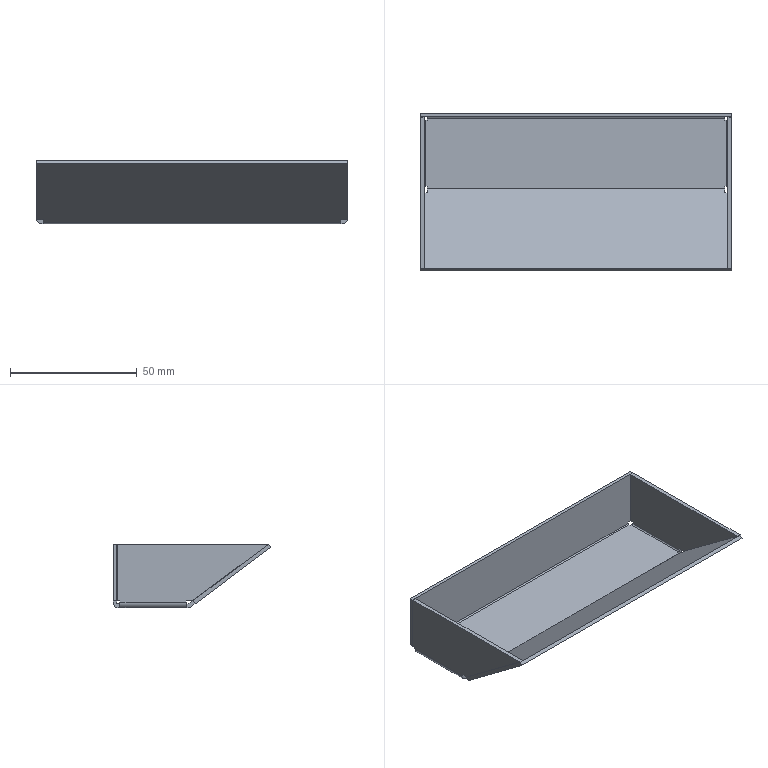Part | STEP file | Rear Closing Plate Handle | 1 solid | 46 faces | box 123 x 62.38 x 25 mm | volume 20088 mm3 | plane 38 | cylinder 8 | commonest cylinder face diameters 1 x4 4 x4
STEP:
#1=CARTESIAN_POINT('',(96.195,-17.121,0.3947));
#2=VERTEX_POINT('',#1);
#3=CARTESIAN_POINT('',(-21.305,-17.121,0.3947));
#4=VERTEX_POINT('',#3);
#5=CARTESIAN_POINT('',(-24.055,-17.121,0.3947));
#6=DIRECTION('',(-1.,0.,0.));
#7=VECTOR('',#6,1000.);
#8=LINE('',#5,#7);
#9=EDGE_CURVE('',#2,#4,#8,.T.);
#10=ORIENTED_EDGE('',*,*,#9,.F.);
#11=CARTESIAN_POINT('',(96.195,-18.621,1.51));
#12=VERTEX_POINT('',#11);
#13=CARTESIAN_POINT('',(96.195,-16.589,0.));
#14=DIRECTION('',(0.,0.8026,-0.5965));
#15=VECTOR('',#14,1000.);
#16=LINE('',#13,#15);
#17=EDGE_CURVE('',#12,#2,#16,.T.);
#18=ORIENTED_EDGE('',*,*,#17,.F.);
#19=CARTESIAN_POINT('',(98.945,-18.621,1.51));
#20=VERTEX_POINT('',#19);
#21=CARTESIAN_POINT('',(-24.055,-18.621,1.51));
#22=DIRECTION('',(-1.,0.,0.));
#23=VECTOR('',#22,1000.);
#24=LINE('',#21,#23);
#25=EDGE_CURVE('',#20,#12,#24,.T.);
#26=ORIENTED_EDGE('',*,*,#25,.F.);
#27=CARTESIAN_POINT('',(98.945,-48.612,23.796));
#28=VERTEX_POINT('',#27);
#29=CARTESIAN_POINT('',(98.945,-16.589,0.));
#30=DIRECTION('',(0.,0.8026,-0.5965));
#31=VECTOR('',#30,1000.);
#32=LINE('',#29,#31);
#33=EDGE_CURVE('',#28,#20,#32,.T.);
#34=ORIENTED_EDGE('',*,*,#33,.F.);
#35=CARTESIAN_POINT('',(-24.055,-48.612,23.796));
#36=VERTEX_POINT('',#35);
#37=CARTESIAN_POINT('',(-24.055,-48.612,23.796));
#38=DIRECTION('',(1.,0.,0.));
#39=VECTOR('',#38,1000.);
#40=LINE('',#37,#39);
#41=EDGE_CURVE('',#36,#28,#40,.T.);
#42=ORIENTED_EDGE('',*,*,#41,.F.);
#43=CARTESIAN_POINT('',(-24.055,-18.621,1.51));
#44=VERTEX_POINT('',#43);
#45=CARTESIAN_POINT('',(-24.055,-16.589,0.));
#46=DIRECTION('',(0.,-0.8026,0.5965));
#47=VECTOR('',#46,1000.);
#48=LINE('',#45,#47);
#49=EDGE_CURVE('',#44,#36,#48,.T.);
#50=ORIENTED_EDGE('',*,*,#49,.F.);
#51=CARTESIAN_POINT('',(-21.305,-18.621,1.51));
#52=VERTEX_POINT('',#51);
#53=CARTESIAN_POINT('',(-24.055,-18.621,1.51));
#54=DIRECTION('',(-1.,0.,0.));
#55=VECTOR('',#54,1000.);
#56=LINE('',#53,#55);
#57=EDGE_CURVE('',#52,#44,#56,.T.);
#58=ORIENTED_EDGE('',*,*,#57,.F.);
#59=CARTESIAN_POINT('',(-21.305,-16.589,0.));
#60=DIRECTION('',(0.,-0.8026,0.5965));
#61=VECTOR('',#60,1000.);
#62=LINE('',#59,#61);
#63=EDGE_CURVE('',#4,#52,#62,.T.);
#64=ORIENTED_EDGE('',*,*,#63,.F.);
#65=EDGE_LOOP('',(#10,#18,#26,#34,#42,#50,#58,#64));
#66=FACE_OUTER_BOUND('',#65,.T.);
#67=CARTESIAN_POINT('',(-24.055,-16.589,0.));
#68=DIRECTION('',(0.,0.5965,0.8026));
#69=DIRECTION('',(0.,-0.8026,0.5965));
#70=AXIS2_PLACEMENT_3D('',#67,#68,#69);
#71=PLANE('',#70);
#72=ADVANCED_FACE('',(#66),#71,.F.);
#73=CARTESIAN_POINT('',(-21.305,-17.727,2.714));
#74=VERTEX_POINT('',#73);
#75=CARTESIAN_POINT('',(-21.305,-16.226,1.599));
#76=VERTEX_POINT('',#75);
#77=CARTESIAN_POINT('',(-21.305,-17.727,2.714));
#78=DIRECTION('',(0.,0.8026,-0.5965));
#79=VECTOR('',#78,1000.);
#80=LINE('',#77,#79);
#81=EDGE_CURVE('',#74,#76,#80,.T.);
#82=ORIENTED_EDGE('',*,*,#81,.T.);
#83=CARTESIAN_POINT('',(-21.305,-15.928,1.5));
#84=VERTEX_POINT('',#83);
#85=CARTESIAN_POINT('',(-21.305,-15.928,2.));
#86=DIRECTION('',(1.,0.,0.));
#87=DIRECTION('',(0.,0.,-1.));
#88=AXIS2_PLACEMENT_3D('',#85,#86,#87);
#89=CIRCLE('',#88,0.5);
#90=EDGE_CURVE('',#76,#84,#89,.T.);
#91=ORIENTED_EDGE('',*,*,#90,.T.);
#92=CARTESIAN_POINT('',(-21.305,-15.178,1.5));
#93=VERTEX_POINT('',#92);
#94=CARTESIAN_POINT('',(-21.305,0.,1.5));
#95=DIRECTION('',(0.,-1.,0.));
#96=VECTOR('',#95,1000.);
#97=LINE('',#94,#96);
#98=EDGE_CURVE('',#93,#84,#97,.T.);
#99=ORIENTED_EDGE('',*,*,#98,.F.);
#100=CARTESIAN_POINT('',(-21.305,-15.178,0.));
#101=VERTEX_POINT('',#100);
#102=CARTESIAN_POINT('',(-21.305,-15.178,245.861));
#103=DIRECTION('',(0.,0.,-1.));
#104=VECTOR('',#103,1000.);
#105=LINE('',#102,#104);
#106=EDGE_CURVE('',#93,#101,#105,.T.);
#107=ORIENTED_EDGE('',*,*,#106,.T.);
#108=CARTESIAN_POINT('',(-21.305,-15.928,0.));
#109=VERTEX_POINT('',#108);
#110=CARTESIAN_POINT('',(-21.305,0.,0.));
#111=DIRECTION('',(0.,-1.,0.));
#112=VECTOR('',#111,1000.);
#113=LINE('',#110,#112);
#114=EDGE_CURVE('',#101,#109,#113,.T.);
#115=ORIENTED_EDGE('',*,*,#114,.T.);
#116=CARTESIAN_POINT('',(-21.305,-15.928,2.));
#117=DIRECTION('',(1.,0.,0.));
#118=DIRECTION('',(0.,0.,-1.));
#119=AXIS2_PLACEMENT_3D('',#116,#117,#118);
#120=CIRCLE('',#119,2.);
#121=EDGE_CURVE('',#4,#109,#120,.T.);
#122=ORIENTED_EDGE('',*,*,#121,.F.);
#123=ORIENTED_EDGE('',*,*,#63,.T.);
#124=CARTESIAN_POINT('',(-21.305,-18.621,1.51));
#125=DIRECTION('',(0.,0.5965,0.8026));
#126=VECTOR('',#125,1000.);
#127=LINE('',#124,#126);
#128=EDGE_CURVE('',#52,#74,#127,.T.);
#129=ORIENTED_EDGE('',*,*,#128,.T.);
#130=EDGE_LOOP('',(#82,#91,#99,#107,#115,#122,#123,#129));
#131=FACE_OUTER_BOUND('',#130,.T.);
#132=CARTESIAN_POINT('',(-21.305,138.317,208.457));
#133=DIRECTION('',(-1.,0.,0.));
#134=DIRECTION('',(0.,0.,1.));
#135=AXIS2_PLACEMENT_3D('',#132,#133,#134);
#136=PLANE('',#135);
#137=ADVANCED_FACE('',(#131),#136,.T.);
#138=CARTESIAN_POINT('',(96.195,-15.928,0.));
#139=VERTEX_POINT('',#138);
#140=CARTESIAN_POINT('',(96.195,-15.928,2.));
#141=DIRECTION('',(-1.,0.,0.));
#142=DIRECTION('',(0.,0.,-1.));
#143=AXIS2_PLACEMENT_3D('',#140,#141,#142);
#144=CIRCLE('',#143,2.);
#145=EDGE_CURVE('',#139,#2,#144,.T.);
#146=ORIENTED_EDGE('',*,*,#145,.T.);
#147=ORIENTED_EDGE('',*,*,#9,.T.);
#148=ORIENTED_EDGE('',*,*,#121,.T.);
#149=CARTESIAN_POINT('',(-164.795,-15.928,0.));
#150=DIRECTION('',(1.,0.,0.));
#151=VECTOR('',#150,1000.);
#152=LINE('',#149,#151);
#153=EDGE_CURVE('',#109,#139,#152,.T.);
#154=ORIENTED_EDGE('',*,*,#153,.T.);
#155=EDGE_LOOP('',(#146,#147,#148,#154));
#156=FACE_OUTER_BOUND('',#155,.T.);
#157=CARTESIAN_POINT('',(-164.795,-15.928,2.));
#158=DIRECTION('',(1.,0.,0.));
#159=DIRECTION('',(0.,0.,-1.));
#160=AXIS2_PLACEMENT_3D('',#157,#158,#159);
#161=CYLINDRICAL_SURFACE('',#160,2.);
#162=ADVANCED_FACE('',(#156),#161,.T.);
#163=CARTESIAN_POINT('',(96.195,-16.226,1.599));
#164=VERTEX_POINT('',#163);
#165=CARTESIAN_POINT('',(96.195,-17.727,2.714));
#166=VERTEX_POINT('',#165);
#167=CARTESIAN_POINT('',(96.195,-16.226,1.599));
#168=DIRECTION('',(0.,-0.8026,0.5965));
#169=VECTOR('',#168,1000.);
#170=LINE('',#167,#169);
#171=EDGE_CURVE('',#164,#166,#170,.T.);
#172=ORIENTED_EDGE('',*,*,#171,.T.);
#173=CARTESIAN_POINT('',(96.195,-17.727,2.714));
#174=DIRECTION('',(0.,-0.5965,-0.8026));
#175=VECTOR('',#174,1000.);
#176=LINE('',#173,#175);
#177=EDGE_CURVE('',#166,#12,#176,.T.);
#178=ORIENTED_EDGE('',*,*,#177,.T.);
#179=ORIENTED_EDGE('',*,*,#17,.T.);
#180=ORIENTED_EDGE('',*,*,#145,.F.);
#181=CARTESIAN_POINT('',(96.195,-15.178,0.));
#182=VERTEX_POINT('',#181);
#183=CARTESIAN_POINT('',(96.195,0.,0.));
#184=DIRECTION('',(0.,1.,0.));
#185=VECTOR('',#184,1000.);
#186=LINE('',#183,#185);
#187=EDGE_CURVE('',#139,#182,#186,.T.);
#188=ORIENTED_EDGE('',*,*,#187,.T.);
#189=CARTESIAN_POINT('',(96.195,-15.178,1.5));
#190=VERTEX_POINT('',#189);
#191=CARTESIAN_POINT('',(96.195,-15.178,245.861));
#192=DIRECTION('',(0.,0.,1.));
#193=VECTOR('',#192,1000.);
#194=LINE('',#191,#193);
#195=EDGE_CURVE('',#182,#190,#194,.T.);
#196=ORIENTED_EDGE('',*,*,#195,.T.);
#197=CARTESIAN_POINT('',(96.195,-15.928,1.5));
#198=VERTEX_POINT('',#197);
#199=CARTESIAN_POINT('',(96.195,0.,1.5));
#200=DIRECTION('',(0.,-1.,0.));
#201=VECTOR('',#200,1000.);
#202=LINE('',#199,#201);
#203=EDGE_CURVE('',#190,#198,#202,.T.);
#204=ORIENTED_EDGE('',*,*,#203,.T.);
#205=CARTESIAN_POINT('',(96.195,-15.928,2.));
#206=DIRECTION('',(-1.,0.,0.));
#207=DIRECTION('',(0.,0.,-1.));
#208=AXIS2_PLACEMENT_3D('',#205,#206,#207);
#209=CIRCLE('',#208,0.5);
#210=EDGE_CURVE('',#198,#164,#209,.T.);
#211=ORIENTED_EDGE('',*,*,#210,.T.);
#212=EDGE_LOOP('',(#172,#178,#179,#180,#188,#196,#204,#211));
#213=FACE_OUTER_BOUND('',#212,.T.);
#214=CARTESIAN_POINT('',(96.195,138.317,208.457));
#215=DIRECTION('',(1.,0.,0.));
#216=DIRECTION('',(0.,0.,-1.));
#217=AXIS2_PLACEMENT_3D('',#214,#215,#216);
#218=PLANE('',#217);
#219=ADVANCED_FACE('',(#213),#218,.T.);
#220=CARTESIAN_POINT('',(98.945,-17.727,2.714));
#221=VERTEX_POINT('',#220);
#222=CARTESIAN_POINT('',(-24.055,-17.727,2.714));
#223=DIRECTION('',(1.,0.,0.));
#224=VECTOR('',#223,1000.);
#225=LINE('',#222,#224);
#226=EDGE_CURVE('',#166,#221,#225,.T.);
#227=ORIENTED_EDGE('',*,*,#226,.T.);
#228=CARTESIAN_POINT('',(98.945,136.285,209.967));
#229=DIRECTION('',(0.,-0.5965,-0.8026));
#230=VECTOR('',#229,1000.);
#231=LINE('',#228,#230);
#232=EDGE_CURVE('',#221,#20,#231,.T.);
#233=ORIENTED_EDGE('',*,*,#232,.T.);
#234=ORIENTED_EDGE('',*,*,#25,.T.);
#235=ORIENTED_EDGE('',*,*,#177,.F.);
#236=EDGE_LOOP('',(#227,#233,#234,#235));
#237=FACE_OUTER_BOUND('',#236,.T.);
#238=CARTESIAN_POINT('',(-24.055,136.285,209.967));
#239=DIRECTION('',(0.,0.8026,-0.5965));
#240=DIRECTION('',(0.,0.5965,0.8026));
#241=AXIS2_PLACEMENT_3D('',#238,#239,#240);
#242=PLANE('',#241);
#243=ADVANCED_FACE('',(#237),#242,.T.);
#244=ORIENTED_EDGE('',*,*,#33,.T.);
#245=ORIENTED_EDGE('',*,*,#232,.F.);
#246=CARTESIAN_POINT('',(98.945,-47.717,25.));
#247=VERTEX_POINT('',#246);
#248=CARTESIAN_POINT('',(98.945,-47.717,25.));
#249=DIRECTION('',(0.,0.8026,-0.5965));
#250=VECTOR('',#249,1000.);
#251=LINE('',#248,#250);
#252=EDGE_CURVE('',#247,#221,#251,.T.);
#253=ORIENTED_EDGE('',*,*,#252,.F.);
#254=CARTESIAN_POINT('',(98.945,-48.612,23.796));
#255=DIRECTION('',(0.,0.5965,0.8026));
#256=VECTOR('',#255,1000.);
#257=LINE('',#254,#256);
#258=EDGE_CURVE('',#28,#247,#257,.T.);
#259=ORIENTED_EDGE('',*,*,#258,.F.);
#260=EDGE_LOOP('',(#244,#245,#253,#259));
#261=FACE_OUTER_BOUND('',#260,.T.);
#262=CARTESIAN_POINT('',(98.945,88.075,245.792));
#263=DIRECTION('',(-1.,0.,0.));
#264=DIRECTION('',(0.,-1.,0.));
#265=AXIS2_PLACEMENT_3D('',#262,#263,#264);
#266=PLANE('',#265);
#267=ADVANCED_FACE('',(#261),#266,.F.);
#268=ORIENTED_EDGE('',*,*,#41,.T.);
#269=ORIENTED_EDGE('',*,*,#258,.T.);
#270=CARTESIAN_POINT('',(-24.055,-47.717,25.));
#271=VERTEX_POINT('',#270);
#272=CARTESIAN_POINT('',(-24.055,-47.717,25.));
#273=DIRECTION('',(1.,0.,0.));
#274=VECTOR('',#273,1000.);
#275=LINE('',#272,#274);
#276=EDGE_CURVE('',#271,#247,#275,.T.);
#277=ORIENTED_EDGE('',*,*,#276,.F.);
#278=CARTESIAN_POINT('',(-24.055,106.295,232.253));
#279=DIRECTION('',(0.,0.5965,0.8026));
#280=VECTOR('',#279,1000.);
#281=LINE('',#278,#280);
#282=EDGE_CURVE('',#36,#271,#281,.T.);
#283=ORIENTED_EDGE('',*,*,#282,.F.);
#284=EDGE_LOOP('',(#268,#269,#277,#283));
#285=FACE_OUTER_BOUND('',#284,.T.);
#286=CARTESIAN_POINT('',(-24.055,106.295,232.253));
#287=DIRECTION('',(0.,0.8026,-0.5965));
#288=DIRECTION('',(0.,0.5965,0.8026));
#289=AXIS2_PLACEMENT_3D('',#286,#287,#288);
#290=PLANE('',#289);
#291=ADVANCED_FACE('',(#285),#290,.F.);
#292=ORIENTED_EDGE('',*,*,#49,.T.);
#293=ORIENTED_EDGE('',*,*,#282,.T.);
#294=CARTESIAN_POINT('',(-24.055,-17.727,2.714));
#295=VERTEX_POINT('',#294);
#296=CARTESIAN_POINT('',(-24.055,-17.727,2.714));
#297=DIRECTION('',(0.,-0.8026,0.5965));
#298=VECTOR('',#297,1000.);
#299=LINE('',#296,#298);
#300=EDGE_CURVE('',#295,#271,#299,.T.);
#301=ORIENTED_EDGE('',*,*,#300,.F.);
#302=CARTESIAN_POINT('',(-24.055,-18.621,1.51));
#303=DIRECTION('',(0.,0.5965,0.8026));
#304=VECTOR('',#303,1000.);
#305=LINE('',#302,#304);
#306=EDGE_CURVE('',#44,#295,#305,.T.);
#307=ORIENTED_EDGE('',*,*,#306,.F.);
#308=EDGE_LOOP('',(#292,#293,#301,#307));
#309=FACE_OUTER_BOUND('',#308,.T.);
#310=CARTESIAN_POINT('',(-24.055,156.138,195.213));
#311=DIRECTION('',(1.,0.,0.));
#312=DIRECTION('',(0.,0.,-1.));
#313=AXIS2_PLACEMENT_3D('',#310,#311,#312);
#314=PLANE('',#313);
#315=ADVANCED_FACE('',(#309),#314,.F.);
#316=CARTESIAN_POINT('',(-24.055,-17.727,2.714));
#317=DIRECTION('',(1.,0.,0.));
#318=VECTOR('',#317,1000.);
#319=LINE('',#316,#318);
#320=EDGE_CURVE('',#295,#74,#319,.T.);
#321=ORIENTED_EDGE('',*,*,#320,.T.);
#322=ORIENTED_EDGE('',*,*,#128,.F.);
#323=ORIENTED_EDGE('',*,*,#57,.T.);
#324=ORIENTED_EDGE('',*,*,#306,.T.);
#325=EDGE_LOOP('',(#321,#322,#323,#324));
#326=FACE_OUTER_BOUND('',#325,.T.);
#327=CARTESIAN_POINT('',(-24.055,136.285,209.967));
#328=DIRECTION('',(0.,0.8026,-0.5965));
#329=DIRECTION('',(0.,0.5965,0.8026));
#330=AXIS2_PLACEMENT_3D('',#327,#328,#329);
#331=PLANE('',#330);
#332=ADVANCED_FACE('',(#326),#331,.T.);
#333=CARTESIAN_POINT('',(-24.055,-16.226,1.599));
#334=DIRECTION('',(-1.,0.,0.));
#335=VECTOR('',#334,1000.);
#336=LINE('',#333,#335);
#337=EDGE_CURVE('',#164,#76,#336,.T.);
#338=ORIENTED_EDGE('',*,*,#337,.T.);
#339=ORIENTED_EDGE('',*,*,#81,.F.);
#340=ORIENTED_EDGE('',*,*,#320,.F.);
#341=ORIENTED_EDGE('',*,*,#300,.T.);
#342=ORIENTED_EDGE('',*,*,#276,.T.);
#343=ORIENTED_EDGE('',*,*,#252,.T.);
#344=ORIENTED_EDGE('',*,*,#226,.F.);
#345=ORIENTED_EDGE('',*,*,#171,.F.);
#346=EDGE_LOOP('',(#338,#339,#340,#341,#342,#343,#344,#345));
#347=FACE_OUTER_BOUND('',#346,.T.);
#348=CARTESIAN_POINT('',(-24.055,-15.695,1.204));
#349=DIRECTION('',(0.,0.5965,0.8026));
#350=DIRECTION('',(0.,-0.8026,0.5965));
#351=AXIS2_PLACEMENT_3D('',#348,#349,#350);
#352=PLANE('',#351);
#353=ADVANCED_FACE('',(#347),#352,.T.);
#354=ORIENTED_EDGE('',*,*,#114,.F.);
#355=CARTESIAN_POINT('',(-22.055,-15.178,0.));
#356=VERTEX_POINT('',#355);
#357=CARTESIAN_POINT('',(0.,-15.178,0.));
#358=DIRECTION('',(1.,0.,0.));
#359=VECTOR('',#358,1000.);
#360=LINE('',#357,#359);
#361=EDGE_CURVE('',#356,#101,#360,.T.);
#362=ORIENTED_EDGE('',*,*,#361,.F.);
#363=CARTESIAN_POINT('',(-22.055,11.018,0.));
#364=VERTEX_POINT('',#363);
#365=CARTESIAN_POINT('',(-22.055,0.,0.));
#366=DIRECTION('',(0.,-1.,0.));
#367=VECTOR('',#366,1000.);
#368=LINE('',#365,#367);
#369=EDGE_CURVE('',#364,#356,#368,.T.);
#370=ORIENTED_EDGE('',*,*,#369,.F.);
#371=CARTESIAN_POINT('',(-21.305,11.018,0.));
#372=VERTEX_POINT('',#371);
#373=CARTESIAN_POINT('',(0.,11.018,0.));
#374=DIRECTION('',(-1.,0.,0.));
#375=VECTOR('',#374,1000.);
#376=LINE('',#373,#375);
#377=EDGE_CURVE('',#372,#364,#376,.T.);
#378=ORIENTED_EDGE('',*,*,#377,.F.);
#379=CARTESIAN_POINT('',(-21.305,11.768,0.));
#380=VERTEX_POINT('',#379);
#381=CARTESIAN_POINT('',(-21.305,0.,0.));
#382=DIRECTION('',(0.,1.,0.));
#383=VECTOR('',#382,1000.);
#384=LINE('',#381,#383);
#385=EDGE_CURVE('',#372,#380,#384,.T.);
#386=ORIENTED_EDGE('',*,*,#385,.T.);
#387=CARTESIAN_POINT('',(96.195,11.768,0.));
#388=VERTEX_POINT('',#387);
#389=CARTESIAN_POINT('',(0.,11.768,0.));
#390=DIRECTION('',(-1.,0.,0.));
#391=VECTOR('',#390,1000.);
#392=LINE('',#389,#391);
#393=EDGE_CURVE('',#388,#380,#392,.T.);
#394=ORIENTED_EDGE('',*,*,#393,.F.);
#395=CARTESIAN_POINT('',(96.195,11.018,0.));
#396=VERTEX_POINT('',#395);
#397=CARTESIAN_POINT('',(96.195,0.,0.));
#398=DIRECTION('',(0.,-1.,0.));
#399=VECTOR('',#398,1000.);
#400=LINE('',#397,#399);
#401=EDGE_CURVE('',#388,#396,#400,.T.);
#402=ORIENTED_EDGE('',*,*,#401,.T.);
#403=CARTESIAN_POINT('',(96.945,11.018,0.));
#404=VERTEX_POINT('',#403);
#405=CARTESIAN_POINT('',(0.,11.018,0.));
#406=DIRECTION('',(-1.,0.,0.));
#407=VECTOR('',#406,1000.);
#408=LINE('',#405,#407);
#409=EDGE_CURVE('',#404,#396,#408,.T.);
#410=ORIENTED_EDGE('',*,*,#409,.F.);
#411=CARTESIAN_POINT('',(96.945,-15.178,0.));
#412=VERTEX_POINT('',#411);
#413=CARTESIAN_POINT('',(96.945,0.,0.));
#414=DIRECTION('',(0.,1.,0.));
#415=VECTOR('',#414,1000.);
#416=LINE('',#413,#415);
#417=EDGE_CURVE('',#412,#404,#416,.T.);
#418=ORIENTED_EDGE('',*,*,#417,.F.);
#419=CARTESIAN_POINT('',(0.,-15.178,0.));
#420=DIRECTION('',(1.,0.,0.));
#421=VECTOR('',#420,1000.);
#422=LINE('',#419,#421);
#423=EDGE_CURVE('',#182,#412,#422,.T.);
#424=ORIENTED_EDGE('',*,*,#423,.F.);
#425=ORIENTED_EDGE('',*,*,#187,.F.);
#426=ORIENTED_EDGE('',*,*,#153,.F.);
#427=EDGE_LOOP('',(#354,#362,#370,#378,#386,#394,#402,#410,#418,#424,#425,#426));
#428=FACE_OUTER_BOUND('',#427,.T.);
#429=CARTESIAN_POINT('',(0.,0.,0.));
#430=DIRECTION('',(0.,0.,1.));
#431=DIRECTION('',(1.,0.,0.));
#432=AXIS2_PLACEMENT_3D('',#429,#430,#431);
#433=PLANE('',#432);
#434=ADVANCED_FACE('',(#428),#433,.F.);
#435=ORIENTED_EDGE('',*,*,#337,.F.);
#436=ORIENTED_EDGE('',*,*,#210,.F.);
#437=CARTESIAN_POINT('',(-164.795,-15.928,1.5));
#438=DIRECTION('',(1.,0.,0.));
#439=VECTOR('',#438,1000.);
#440=LINE('',#437,#439);
#441=EDGE_CURVE('',#84,#198,#440,.T.);
#442=ORIENTED_EDGE('',*,*,#441,.F.);
#443=ORIENTED_EDGE('',*,*,#90,.F.);
#444=EDGE_LOOP('',(#435,#436,#442,#443));
#445=FACE_OUTER_BOUND('',#444,.T.);
#446=CARTESIAN_POINT('',(-164.795,-15.928,2.));
#447=DIRECTION('',(1.,0.,0.));
#448=DIRECTION('',(0.,0.,-1.));
#449=AXIS2_PLACEMENT_3D('',#446,#447,#448);
#450=CYLINDRICAL_SURFACE('',#449,0.5);
#451=ADVANCED_FACE('',(#445),#450,.F.);
#452=CARTESIAN_POINT('',(-22.055,-15.178,1.5));
#453=VERTEX_POINT('',#452);
#454=CARTESIAN_POINT('',(0.,-15.178,1.5));
#455=DIRECTION('',(-1.,0.,0.));
#456=VECTOR('',#455,1000.);
#457=LINE('',#454,#456);
#458=EDGE_CURVE('',#93,#453,#457,.T.);
#459=ORIENTED_EDGE('',*,*,#458,.T.);
#460=CARTESIAN_POINT('',(-22.555,-15.178,2.));
#461=VERTEX_POINT('',#460);
#462=CARTESIAN_POINT('',(-22.055,-15.178,2.));
#463=DIRECTION('',(0.,1.,0.));
#464=DIRECTION('',(0.,0.,-1.));
#465=AXIS2_PLACEMENT_3D('',#462,#463,#464);
#466=CIRCLE('',#465,0.5);
#467=EDGE_CURVE('',#453,#461,#466,.T.);
#468=ORIENTED_EDGE('',*,*,#467,.T.);
#469=CARTESIAN_POINT('',(-22.555,-15.178,2.75));
#470=VERTEX_POINT('',#469);
#471=CARTESIAN_POINT('',(-22.555,-15.178,25.));
#472=DIRECTION('',(0.,0.,1.));
#473=VECTOR('',#472,1000.);
#474=LINE('',#471,#473);
#475=EDGE_CURVE('',#461,#470,#474,.T.);
#476=ORIENTED_EDGE('',*,*,#475,.T.);
#477=CARTESIAN_POINT('',(-24.055,-15.178,2.75));
#478=VERTEX_POINT('',#477);
#479=CARTESIAN_POINT('',(105.432,-15.178,2.75));
#480=DIRECTION('',(1.,0.,0.));
#481=VECTOR('',#480,1000.);
#482=LINE('',#479,#481);
#483=EDGE_CURVE('',#478,#470,#482,.T.);
#484=ORIENTED_EDGE('',*,*,#483,.F.);
#485=CARTESIAN_POINT('',(-24.055,-15.178,2.));
#486=VERTEX_POINT('',#485);
#487=CARTESIAN_POINT('',(-24.055,-15.178,25.));
#488=DIRECTION('',(0.,0.,-1.));
#489=VECTOR('',#488,1000.);
#490=LINE('',#487,#489);
#491=EDGE_CURVE('',#478,#486,#490,.T.);
#492=ORIENTED_EDGE('',*,*,#491,.T.);
#493=CARTESIAN_POINT('',(-22.055,-15.178,2.));
#494=DIRECTION('',(0.,1.,0.));
#495=DIRECTION('',(0.,0.,-1.));
#496=AXIS2_PLACEMENT_3D('',#493,#494,#495);
#497=CIRCLE('',#496,2.);
#498=EDGE_CURVE('',#356,#486,#497,.T.);
#499=ORIENTED_EDGE('',*,*,#498,.F.);
#500=ORIENTED_EDGE('',*,*,#361,.T.);
#501=ORIENTED_EDGE('',*,*,#106,.F.);
#502=EDGE_LOOP('',(#459,#468,#476,#484,#492,#499,#500,#501));
#503=FACE_OUTER_BOUND('',#502,.T.);
#504=CARTESIAN_POINT('',(0.,-15.178,245.861));
#505=DIRECTION('',(0.,-1.,0.));
#506=DIRECTION('',(1.,0.,0.));
#507=AXIS2_PLACEMENT_3D('',#504,#505,#506);
#508=PLANE('',#507);
#509=ADVANCED_FACE('',(#503),#508,.T.);
#510=ORIENTED_EDGE('',*,*,#498,.T.);
#511=CARTESIAN_POINT('',(-24.055,11.018,2.));
#512=VERTEX_POINT('',#511);
#513=CARTESIAN_POINT('',(-24.055,174.2,2.));
#514=DIRECTION('',(0.,1.,0.));
#515=VECTOR('',#514,1000.);
#516=LINE('',#513,#515);
#517=EDGE_CURVE('',#486,#512,#516,.T.);
#518=ORIENTED_EDGE('',*,*,#517,.T.);
#519=CARTESIAN_POINT('',(-22.055,11.018,2.));
#520=DIRECTION('',(0.,-1.,0.));
#521=DIRECTION('',(0.,0.,-1.));
#522=AXIS2_PLACEMENT_3D('',#519,#520,#521);
#523=CIRCLE('',#522,2.);
#524=EDGE_CURVE('',#512,#364,#523,.T.);
#525=ORIENTED_EDGE('',*,*,#524,.T.);
#526=ORIENTED_EDGE('',*,*,#369,.T.);
#527=EDGE_LOOP('',(#510,#518,#525,#526));
#528=FACE_OUTER_BOUND('',#527,.T.);
#529=CARTESIAN_POINT('',(-22.055,174.2,2.));
#530=DIRECTION('',(0.,-1.,0.));
#531=DIRECTION('',(0.,0.,-1.));
#532=AXIS2_PLACEMENT_3D('',#529,#530,#531);
#533=CYLINDRICAL_SURFACE('',#532,2.);
#534=ADVANCED_FACE('',(#528),#533,.T.);
#535=ORIENTED_EDGE('',*,*,#377,.T.);
#536=ORIENTED_EDGE('',*,*,#524,.F.);
#537=CARTESIAN_POINT('',(-24.055,11.018,2.75));
#538=VERTEX_POINT('',#537);
#539=CARTESIAN_POINT('',(-24.055,11.018,25.));
#540=DIRECTION('',(0.,0.,1.));
#541=VECTOR('',#540,1000.);
#542=LINE('',#539,#541);
#543=EDGE_CURVE('',#512,#538,#542,.T.);
#544=ORIENTED_EDGE('',*,*,#543,.T.);
#545=CARTESIAN_POINT('',(-22.555,11.018,2.75));
#546=VERTEX_POINT('',#545);
#547=CARTESIAN_POINT('',(105.432,11.018,2.75));
#548=DIRECTION('',(-1.,0.,0.));
#549=VECTOR('',#548,1000.);
#550=LINE('',#547,#549);
#551=EDGE_CURVE('',#546,#538,#550,.T.);
#552=ORIENTED_EDGE('',*,*,#551,.F.);
#553=CARTESIAN_POINT('',(-22.555,11.018,2.));
#554=VERTEX_POINT('',#553);
#555=CARTESIAN_POINT('',(-22.555,11.018,25.));
#556=DIRECTION('',(0.,0.,1.));
#557=VECTOR('',#556,1000.);
#558=LINE('',#555,#557);
#559=EDGE_CURVE('',#554,#546,#558,.T.);
#560=ORIENTED_EDGE('',*,*,#559,.F.);
#561=CARTESIAN_POINT('',(-22.055,11.018,1.5));
#562=VERTEX_POINT('',#561);
#563=CARTESIAN_POINT('',(-22.055,11.018,2.));
#564=DIRECTION('',(0.,-1.,0.));
#565=DIRECTION('',(0.,0.,-1.));
#566=AXIS2_PLACEMENT_3D('',#563,#564,#565);
#567=CIRCLE('',#566,0.5);
#568=EDGE_CURVE('',#554,#562,#567,.T.);
#569=ORIENTED_EDGE('',*,*,#568,.T.);
#570=CARTESIAN_POINT('',(-21.305,11.018,1.5));
#571=VERTEX_POINT('',#570);
#572=CARTESIAN_POINT('',(0.,11.018,1.5));
#573=DIRECTION('',(-1.,0.,0.));
#574=VECTOR('',#573,1000.);
#575=LINE('',#572,#574);
#576=EDGE_CURVE('',#571,#562,#575,.T.);
#577=ORIENTED_EDGE('',*,*,#576,.F.);
#578=CARTESIAN_POINT('',(-21.305,11.018,245.861));
#579=DIRECTION('',(0.,0.,1.));
#580=VECTOR('',#579,1000.);
#581=LINE('',#578,#580);
#582=EDGE_CURVE('',#372,#571,#581,.T.);
#583=ORIENTED_EDGE('',*,*,#582,.F.);
#584=EDGE_LOOP('',(#535,#536,#544,#552,#560,#569,#577,#583));
#585=FACE_OUTER_BOUND('',#584,.T.);
#586=CARTESIAN_POINT('',(0.,11.018,245.861));
#587=DIRECTION('',(0.,-1.,0.));
#588=DIRECTION('',(0.,0.,-1.));
#589=AXIS2_PLACEMENT_3D('',#586,#587,#588);
#590=PLANE('',#589);
#591=ADVANCED_FACE('',(#585),#590,.F.);
#592=CARTESIAN_POINT('',(-21.305,13.768,2.));
#593=VERTEX_POINT('',#592);
#594=CARTESIAN_POINT('',(-21.305,11.768,2.));
#595=DIRECTION('',(1.,0.,0.));
#596=DIRECTION('',(0.,0.,1.));
#597=AXIS2_PLACEMENT_3D('',#594,#595,#596);
#598=CIRCLE('',#597,2.);
#599=EDGE_CURVE('',#380,#593,#598,.T.);
#600=ORIENTED_EDGE('',*,*,#599,.T.);
#601=CARTESIAN_POINT('',(96.195,13.768,2.));
#602=VERTEX_POINT('',#601);
#603=CARTESIAN_POINT('',(287.743,13.768,2.));
#604=DIRECTION('',(1.,0.,0.));
#605=VECTOR('',#604,1000.);
#606=LINE('',#603,#605);
#607=EDGE_CURVE('',#593,#602,#606,.T.);
#608=ORIENTED_EDGE('',*,*,#607,.T.);
#609=CARTESIAN_POINT('',(96.195,11.768,2.));
#610=DIRECTION('',(-1.,0.,0.));
#611=DIRECTION('',(0.,0.,1.));
#612=AXIS2_PLACEMENT_3D('',#609,#610,#611);
#613=CIRCLE('',#612,2.);
#614=EDGE_CURVE('',#602,#388,#613,.T.);
#615=ORIENTED_EDGE('',*,*,#614,.T.);
#616=ORIENTED_EDGE('',*,*,#393,.T.);
#617=EDGE_LOOP('',(#600,#608,#615,#616));
#618=FACE_OUTER_BOUND('',#617,.T.);
#619=CARTESIAN_POINT('',(287.743,11.768,2.));
#620=DIRECTION('',(-1.,0.,0.));
#621=DIRECTION('',(0.,0.,1.));
#622=AXIS2_PLACEMENT_3D('',#619,#620,#621);
#623=CYLINDRICAL_SURFACE('',#622,2.);
#624=ADVANCED_FACE('',(#618),#623,.T.);
#625=ORIENTED_EDGE('',*,*,#409,.T.);
#626=CARTESIAN_POINT('',(96.195,11.018,1.5));
#627=VERTEX_POINT('',#626);
#628=CARTESIAN_POINT('',(96.195,11.018,245.861));
#629=DIRECTION('',(0.,0.,-1.));
#630=VECTOR('',#629,1000.);
#631=LINE('',#628,#630);
#632=EDGE_CURVE('',#627,#396,#631,.T.);
#633=ORIENTED_EDGE('',*,*,#632,.F.);
#634=CARTESIAN_POINT('',(96.945,11.018,1.5));
#635=VERTEX_POINT('',#634);
#636=CARTESIAN_POINT('',(0.,11.018,1.5));
#637=DIRECTION('',(-1.,0.,0.));
#638=VECTOR('',#637,1000.);
#639=LINE('',#636,#638);
#640=EDGE_CURVE('',#635,#627,#639,.T.);
#641=ORIENTED_EDGE('',*,*,#640,.F.);
#642=CARTESIAN_POINT('',(97.445,11.018,2.));
#643=VERTEX_POINT('',#642);
#644=CARTESIAN_POINT('',(96.945,11.018,2.));
#645=DIRECTION('',(0.,-1.,0.));
#646=DIRECTION('',(0.,0.,1.));
#647=AXIS2_PLACEMENT_3D('',#644,#645,#646);
#648=CIRCLE('',#647,0.5);
#649=EDGE_CURVE('',#635,#643,#648,.T.);
#650=ORIENTED_EDGE('',*,*,#649,.T.);
#651=CARTESIAN_POINT('',(97.445,11.018,2.75));
#652=VERTEX_POINT('',#651);
#653=CARTESIAN_POINT('',(97.445,11.018,25.));
#654=DIRECTION('',(0.,0.,-1.));
#655=VECTOR('',#654,1000.);
#656=LINE('',#653,#655);
#657=EDGE_CURVE('',#652,#643,#656,.T.);
#658=ORIENTED_EDGE('',*,*,#657,.F.);
#659=CARTESIAN_POINT('',(98.945,11.018,2.75));
#660=VERTEX_POINT('',#659);
#661=CARTESIAN_POINT('',(-30.542,11.018,2.75));
#662=DIRECTION('',(-1.,0.,0.));
#663=VECTOR('',#662,1000.);
#664=LINE('',#661,#663);
#665=EDGE_CURVE('',#660,#652,#664,.T.);
#666=ORIENTED_EDGE('',*,*,#665,.F.);
#667=CARTESIAN_POINT('',(98.945,11.018,2.));
#668=VERTEX_POINT('',#667);
#669=CARTESIAN_POINT('',(98.945,11.018,25.));
#670=DIRECTION('',(0.,0.,-1.));
#671=VECTOR('',#670,1000.);
#672=LINE('',#669,#671);
#673=EDGE_CURVE('',#660,#668,#672,.T.);
#674=ORIENTED_EDGE('',*,*,#673,.T.);
#675=CARTESIAN_POINT('',(96.945,11.018,2.));
#676=DIRECTION('',(0.,-1.,0.));
#677=DIRECTION('',(0.,0.,1.));
#678=AXIS2_PLACEMENT_3D('',#675,#676,#677);
#679=CIRCLE('',#678,2.);
#680=EDGE_CURVE('',#404,#668,#679,.T.);
#681=ORIENTED_EDGE('',*,*,#680,.F.);
#682=EDGE_LOOP('',(#625,#633,#641,#650,#658,#666,#674,#681));
#683=FACE_OUTER_BOUND('',#682,.T.);
#684=CARTESIAN_POINT('',(0.,11.018,245.861));
#685=DIRECTION('',(0.,-1.,0.));
#686=DIRECTION('',(0.,0.,-1.));
#687=AXIS2_PLACEMENT_3D('',#684,#685,#686);
#688=PLANE('',#687);
#689=ADVANCED_FACE('',(#683),#688,.F.);
#690=ORIENTED_EDGE('',*,*,#680,.T.);
#691=CARTESIAN_POINT('',(98.945,-15.178,2.));
#692=VERTEX_POINT('',#691);
#693=CARTESIAN_POINT('',(98.945,-198.697,2.));
#694=DIRECTION('',(0.,-1.,0.));
#695=VECTOR('',#694,1000.);
#696=LINE('',#693,#695);
#697=EDGE_CURVE('',#668,#692,#696,.T.);
#698=ORIENTED_EDGE('',*,*,#697,.T.);
#699=CARTESIAN_POINT('',(96.945,-15.178,2.));
#700=DIRECTION('',(0.,1.,0.));
#701=DIRECTION('',(0.,0.,1.));
#702=AXIS2_PLACEMENT_3D('',#699,#700,#701);
#703=CIRCLE('',#702,2.);
#704=EDGE_CURVE('',#692,#412,#703,.T.);
#705=ORIENTED_EDGE('',*,*,#704,.T.);
#706=ORIENTED_EDGE('',*,*,#417,.T.);
#707=EDGE_LOOP('',(#690,#698,#705,#706));
#708=FACE_OUTER_BOUND('',#707,.T.);
#709=CARTESIAN_POINT('',(96.945,-198.697,2.));
#710=DIRECTION('',(0.,1.,0.));
#711=DIRECTION('',(0.,0.,1.));
#712=AXIS2_PLACEMENT_3D('',#709,#710,#711);
#713=CYLINDRICAL_SURFACE('',#712,2.);
#714=ADVANCED_FACE('',(#708),#713,.T.);
#715=CARTESIAN_POINT('',(96.945,-15.178,1.5));
#716=VERTEX_POINT('',#715);
#717=CARTESIAN_POINT('',(0.,-15.178,1.5));
#718=DIRECTION('',(-1.,0.,0.));
#719=VECTOR('',#718,1000.);
#720=LINE('',#717,#719);
#721=EDGE_CURVE('',#716,#190,#720,.T.);
#722=ORIENTED_EDGE('',*,*,#721,.T.);
#723=ORIENTED_EDGE('',*,*,#195,.F.);
#724=ORIENTED_EDGE('',*,*,#423,.T.);
#725=ORIENTED_EDGE('',*,*,#704,.F.);
#726=CARTESIAN_POINT('',(98.945,-15.178,2.75));
#727=VERTEX_POINT('',#726);
#728=CARTESIAN_POINT('',(98.945,-15.178,25.));
#729=DIRECTION('',(0.,0.,1.));
#730=VECTOR('',#729,1000.);
#731=LINE('',#728,#730);
#732=EDGE_CURVE('',#692,#727,#731,.T.);
#733=ORIENTED_EDGE('',*,*,#732,.T.);
#734=CARTESIAN_POINT('',(97.445,-15.178,2.75));
#735=VERTEX_POINT('',#734);
#736=CARTESIAN_POINT('',(-30.542,-15.178,2.75));
#737=DIRECTION('',(1.,0.,0.));
#738=VECTOR('',#737,1000.);
#739=LINE('',#736,#738);
#740=EDGE_CURVE('',#735,#727,#739,.T.);
#741=ORIENTED_EDGE('',*,*,#740,.F.);
#742=CARTESIAN_POINT('',(97.445,-15.178,2.));
#743=VERTEX_POINT('',#742);
#744=CARTESIAN_POINT('',(97.445,-15.178,25.));
#745=DIRECTION('',(0.,0.,-1.));
#746=VECTOR('',#745,1000.);
#747=LINE('',#744,#746);
#748=EDGE_CURVE('',#735,#743,#747,.T.);
#749=ORIENTED_EDGE('',*,*,#748,.T.);
#750=CARTESIAN_POINT('',(96.945,-15.178,2.));
#751=DIRECTION('',(0.,1.,0.));
#752=DIRECTION('',(0.,0.,1.));
#753=AXIS2_PLACEMENT_3D('',#750,#751,#752);
#754=CIRCLE('',#753,0.5);
#755=EDGE_CURVE('',#743,#716,#754,.T.);
#756=ORIENTED_EDGE('',*,*,#755,.T.);
#757=EDGE_LOOP('',(#722,#723,#724,#725,#733,#741,#749,#756));
#758=FACE_OUTER_BOUND('',#757,.T.);
#759=CARTESIAN_POINT('',(0.,-15.178,245.861));
#760=DIRECTION('',(0.,-1.,0.));
#761=DIRECTION('',(0.,0.,-1.));
#762=AXIS2_PLACEMENT_3D('',#759,#760,#761);
#763=PLANE('',#762);
#764=ADVANCED_FACE('',(#758),#763,.T.);
#765=CARTESIAN_POINT('',(-22.055,0.,1.5));
#766=DIRECTION('',(0.,-1.,0.));
#767=VECTOR('',#766,1000.);
#768=LINE('',#765,#767);
#769=EDGE_CURVE('',#562,#453,#768,.T.);
#770=ORIENTED_EDGE('',*,*,#769,.T.);
#771=ORIENTED_EDGE('',*,*,#458,.F.);
#772=ORIENTED_EDGE('',*,*,#98,.T.);
#773=ORIENTED_EDGE('',*,*,#441,.T.);
#774=ORIENTED_EDGE('',*,*,#203,.F.);
#775=ORIENTED_EDGE('',*,*,#721,.F.);
#776=CARTESIAN_POINT('',(96.945,0.,1.5));
#777=DIRECTION('',(0.,1.,0.));
#778=VECTOR('',#777,1000.);
#779=LINE('',#776,#778);
#780=EDGE_CURVE('',#716,#635,#779,.T.);
#781=ORIENTED_EDGE('',*,*,#780,.T.);
#782=ORIENTED_EDGE('',*,*,#640,.T.);
#783=CARTESIAN_POINT('',(96.195,11.768,1.5));
#784=VERTEX_POINT('',#783);
#785=CARTESIAN_POINT('',(96.195,0.,1.5));
#786=DIRECTION('',(0.,1.,0.));
#787=VECTOR('',#786,1000.);
#788=LINE('',#785,#787);
#789=EDGE_CURVE('',#627,#784,#788,.T.);
#790=ORIENTED_EDGE('',*,*,#789,.T.);
#791=CARTESIAN_POINT('',(-21.305,11.768,1.5));
#792=VERTEX_POINT('',#791);
#793=CARTESIAN_POINT('',(0.,11.768,1.5));
#794=DIRECTION('',(-1.,0.,0.));
#795=VECTOR('',#794,1000.);
#796=LINE('',#793,#795);
#797=EDGE_CURVE('',#784,#792,#796,.T.);
#798=ORIENTED_EDGE('',*,*,#797,.T.);
#799=CARTESIAN_POINT('',(-21.305,0.,1.5));
#800=DIRECTION('',(0.,-1.,0.));
#801=VECTOR('',#800,1000.);
#802=LINE('',#799,#801);
#803=EDGE_CURVE('',#792,#571,#802,.T.);
#804=ORIENTED_EDGE('',*,*,#803,.T.);
#805=ORIENTED_EDGE('',*,*,#576,.T.);
#806=EDGE_LOOP('',(#770,#771,#772,#773,#774,#775,#781,#782,#790,#798,#804,#805));
#807=FACE_OUTER_BOUND('',#806,.T.);
#808=CARTESIAN_POINT('',(0.,0.,1.5));
#809=DIRECTION('',(0.,0.,1.));
#810=DIRECTION('',(1.,0.,0.));
#811=AXIS2_PLACEMENT_3D('',#808,#809,#810);
#812=PLANE('',#811);
#813=ADVANCED_FACE('',(#807),#812,.T.);
#814=ORIENTED_EDGE('',*,*,#517,.F.);
#815=ORIENTED_EDGE('',*,*,#491,.F.);
#816=CARTESIAN_POINT('',(-24.055,-17.608,2.75));
#817=VERTEX_POINT('',#816);
#818=CARTESIAN_POINT('',(-24.055,13.768,2.75));
#819=DIRECTION('',(0.,1.,0.));
#820=VECTOR('',#819,1000.);
#821=LINE('',#818,#820);
#822=EDGE_CURVE('',#817,#478,#821,.T.);
#823=ORIENTED_EDGE('',*,*,#822,.F.);
#824=CARTESIAN_POINT('',(-24.055,-47.549,25.));
#825=VERTEX_POINT('',#824);
#826=CARTESIAN_POINT('',(-24.055,-47.549,25.));
#827=DIRECTION('',(0.,0.8026,-0.5965));
#828=VECTOR('',#827,1000.);
#829=LINE('',#826,#828);
#830=EDGE_CURVE('',#825,#817,#829,.T.);
#831=ORIENTED_EDGE('',*,*,#830,.F.);
#832=CARTESIAN_POINT('',(-24.055,12.168,25.));
#833=VERTEX_POINT('',#832);
#834=CARTESIAN_POINT('',(-24.055,13.768,25.));
#835=DIRECTION('',(0.,-1.,0.));
#836=VECTOR('',#835,1000.);
#837=LINE('',#834,#836);
#838=EDGE_CURVE('',#833,#825,#837,.T.);
#839=ORIENTED_EDGE('',*,*,#838,.F.);
#840=CARTESIAN_POINT('',(-24.055,12.168,2.75));
#841=VERTEX_POINT('',#840);
#842=CARTESIAN_POINT('',(-24.055,12.168,25.));
#843=DIRECTION('',(0.,0.,1.));
#844=VECTOR('',#843,1000.);
#845=LINE('',#842,#844);
#846=EDGE_CURVE('',#841,#833,#845,.T.);
#847=ORIENTED_EDGE('',*,*,#846,.F.);
#848=CARTESIAN_POINT('',(-24.055,13.768,2.75));
#849=DIRECTION('',(0.,1.,0.));
#850=VECTOR('',#849,1000.);
#851=LINE('',#848,#850);
#852=EDGE_CURVE('',#538,#841,#851,.T.);
#853=ORIENTED_EDGE('',*,*,#852,.F.);
#854=ORIENTED_EDGE('',*,*,#543,.F.);
#855=EDGE_LOOP('',(#814,#815,#823,#831,#839,#847,#853,#854));
#856=FACE_OUTER_BOUND('',#855,.T.);
#857=CARTESIAN_POINT('',(-24.055,13.768,25.));
#858=DIRECTION('',(1.,0.,0.));
#859=DIRECTION('',(0.,1.,0.));
#860=AXIS2_PLACEMENT_3D('',#857,#858,#859);
#861=PLANE('',#860);
#862=ADVANCED_FACE('',(#856),#861,.F.);
#863=ORIENTED_EDGE('',*,*,#385,.F.);
#864=ORIENTED_EDGE('',*,*,#582,.T.);
#865=ORIENTED_EDGE('',*,*,#803,.F.);
#866=CARTESIAN_POINT('',(-21.305,12.268,2.));
#867=VERTEX_POINT('',#866);
#868=CARTESIAN_POINT('',(-21.305,11.768,2.));
#869=DIRECTION('',(1.,0.,0.));
#870=DIRECTION('',(0.,0.,1.));
#871=AXIS2_PLACEMENT_3D('',#868,#869,#870);
#872=CIRCLE('',#871,0.5);
#873=EDGE_CURVE('',#792,#867,#872,.T.);
#874=ORIENTED_EDGE('',*,*,#873,.T.);
#875=CARTESIAN_POINT('',(-21.305,12.268,2.75));
#876=VERTEX_POINT('',#875);
#877=CARTESIAN_POINT('',(-21.305,12.268,25.));
#878=DIRECTION('',(0.,0.,-1.));
#879=VECTOR('',#878,1000.);
#880=LINE('',#877,#879);
#881=EDGE_CURVE('',#876,#867,#880,.T.);
#882=ORIENTED_EDGE('',*,*,#881,.F.);
#883=CARTESIAN_POINT('',(-21.305,13.768,2.75));
#884=VERTEX_POINT('',#883);
#885=CARTESIAN_POINT('',(-21.305,-237.996,2.75));
#886=DIRECTION('',(0.,-1.,0.));
#887=VECTOR('',#886,1000.);
#888=LINE('',#885,#887);
#889=EDGE_CURVE('',#884,#876,#888,.T.);
#890=ORIENTED_EDGE('',*,*,#889,.F.);
#891=CARTESIAN_POINT('',(-21.305,13.768,25.));
#892=DIRECTION('',(0.,0.,-1.));
#893=VECTOR('',#892,1000.);
#894=LINE('',#891,#893);
#895=EDGE_CURVE('',#884,#593,#894,.T.);
#896=ORIENTED_EDGE('',*,*,#895,.T.);
#897=ORIENTED_EDGE('',*,*,#599,.F.);
#898=EDGE_LOOP('',(#863,#864,#865,#874,#882,#890,#896,#897));
#899=FACE_OUTER_BOUND('',#898,.T.);
#900=CARTESIAN_POINT('',(-21.305,0.,245.861));
#901=DIRECTION('',(1.,0.,0.));
#902=DIRECTION('',(0.,0.,-1.));
#903=AXIS2_PLACEMENT_3D('',#900,#901,#902);
#904=PLANE('',#903);
#905=ADVANCED_FACE('',(#899),#904,.F.);
#906=ORIENTED_EDGE('',*,*,#607,.F.);
#907=ORIENTED_EDGE('',*,*,#895,.F.);
#908=CARTESIAN_POINT('',(-24.055,13.768,2.75));
#909=VERTEX_POINT('',#908);
#910=CARTESIAN_POINT('',(-24.055,13.768,2.75));
#911=DIRECTION('',(1.,0.,0.));
#912=VECTOR('',#911,1000.);
#913=LINE('',#910,#912);
#914=EDGE_CURVE('',#909,#884,#913,.T.);
#915=ORIENTED_EDGE('',*,*,#914,.F.);
#916=CARTESIAN_POINT('',(-24.055,13.768,25.));
#917=VERTEX_POINT('',#916);
#918=CARTESIAN_POINT('',(-24.055,13.768,25.));
#919=DIRECTION('',(0.,0.,-1.));
#920=VECTOR('',#919,1000.);
#921=LINE('',#918,#920);
#922=EDGE_CURVE('',#917,#909,#921,.T.);
#923=ORIENTED_EDGE('',*,*,#922,.F.);
#924=CARTESIAN_POINT('',(98.945,13.768,25.));
#925=VERTEX_POINT('',#924);
#926=CARTESIAN_POINT('',(-24.055,13.768,25.));
#927=DIRECTION('',(-1.,0.,0.));
#928=VECTOR('',#927,1000.);
#929=LINE('',#926,#928);
#930=EDGE_CURVE('',#925,#917,#929,.T.);
#931=ORIENTED_EDGE('',*,*,#930,.F.);
#932=CARTESIAN_POINT('',(98.945,13.768,2.75));
#933=VERTEX_POINT('',#932);
#934=CARTESIAN_POINT('',(98.945,13.768,25.));
#935=DIRECTION('',(0.,0.,1.));
#936=VECTOR('',#935,1000.);
#937=LINE('',#934,#936);
#938=EDGE_CURVE('',#933,#925,#937,.T.);
#939=ORIENTED_EDGE('',*,*,#938,.F.);
#940=CARTESIAN_POINT('',(96.195,13.768,2.75));
#941=VERTEX_POINT('',#940);
#942=CARTESIAN_POINT('',(-24.055,13.768,2.75));
#943=DIRECTION('',(1.,0.,0.));
#944=VECTOR('',#943,1000.);
#945=LINE('',#942,#944);
#946=EDGE_CURVE('',#941,#933,#945,.T.);
#947=ORIENTED_EDGE('',*,*,#946,.F.);
#948=CARTESIAN_POINT('',(96.195,13.768,25.));
#949=DIRECTION('',(0.,0.,-1.));
#950=VECTOR('',#949,1000.);
#951=LINE('',#948,#950);
#952=EDGE_CURVE('',#941,#602,#951,.T.);
#953=ORIENTED_EDGE('',*,*,#952,.T.);
#954=EDGE_LOOP('',(#906,#907,#915,#923,#931,#939,#947,#953));
#955=FACE_OUTER_BOUND('',#954,.T.);
#956=CARTESIAN_POINT('',(-24.055,13.768,25.));
#957=DIRECTION('',(0.,-1.,0.));
#958=DIRECTION('',(0.,0.,-1.));
#959=AXIS2_PLACEMENT_3D('',#956,#957,#958);
#960=PLANE('',#959);
#961=ADVANCED_FACE('',(#955),#960,.F.);
#962=CARTESIAN_POINT('',(96.195,12.268,2.));
#963=VERTEX_POINT('',#962);
#964=CARTESIAN_POINT('',(96.195,11.768,2.));
#965=DIRECTION('',(-1.,0.,0.));
#966=DIRECTION('',(0.,0.,1.));
#967=AXIS2_PLACEMENT_3D('',#964,#965,#966);
#968=CIRCLE('',#967,0.5);
#969=EDGE_CURVE('',#963,#784,#968,.T.);
#970=ORIENTED_EDGE('',*,*,#969,.T.);
#971=ORIENTED_EDGE('',*,*,#789,.F.);
#972=ORIENTED_EDGE('',*,*,#632,.T.);
#973=ORIENTED_EDGE('',*,*,#401,.F.);
#974=ORIENTED_EDGE('',*,*,#614,.F.);
#975=ORIENTED_EDGE('',*,*,#952,.F.);
#976=CARTESIAN_POINT('',(96.195,12.268,2.75));
#977=VERTEX_POINT('',#976);
#978=CARTESIAN_POINT('',(96.195,-237.996,2.75));
#979=DIRECTION('',(0.,1.,0.));
#980=VECTOR('',#979,1000.);
#981=LINE('',#978,#980);
#982=EDGE_CURVE('',#977,#941,#981,.T.);
#983=ORIENTED_EDGE('',*,*,#982,.F.);
#984=CARTESIAN_POINT('',(96.195,12.268,25.));
#985=DIRECTION('',(0.,0.,1.));
#986=VECTOR('',#985,1000.);
#987=LINE('',#984,#986);
#988=EDGE_CURVE('',#963,#977,#987,.T.);
#989=ORIENTED_EDGE('',*,*,#988,.F.);
#990=EDGE_LOOP('',(#970,#971,#972,#973,#974,#975,#983,#989));
#991=FACE_OUTER_BOUND('',#990,.T.);
#992=CARTESIAN_POINT('',(96.195,11.768,2.));
#993=DIRECTION('',(1.,0.,0.));
#994=DIRECTION('',(0.,0.,-1.));
#995=AXIS2_PLACEMENT_3D('',#992,#993,#994);
#996=PLANE('',#995);
#997=ADVANCED_FACE('',(#991),#996,.T.);
#998=ORIENTED_EDGE('',*,*,#697,.F.);
#999=ORIENTED_EDGE('',*,*,#673,.F.);
#1000=CARTESIAN_POINT('',(98.945,12.168,2.75));
#1001=VERTEX_POINT('',#1000);
#1002=CARTESIAN_POINT('',(98.945,13.768,2.75));
#1003=DIRECTION('',(0.,-1.,0.));
#1004=VECTOR('',#1003,1000.);
#1005=LINE('',#1002,#1004);
#1006=EDGE_CURVE('',#1001,#660,#1005,.T.);
#1007=ORIENTED_EDGE('',*,*,#1006,.F.);
#1008=CARTESIAN_POINT('',(98.945,12.168,25.));
#1009=VERTEX_POINT('',#1008);
#1010=CARTESIAN_POINT('',(98.945,12.168,25.));
#1011=DIRECTION('',(0.,0.,-1.));
#1012=VECTOR('',#1011,1000.);
#1013=LINE('',#1010,#1012);
#1014=EDGE_CURVE('',#1009,#1001,#1013,.T.);
#1015=ORIENTED_EDGE('',*,*,#1014,.F.);
#1016=CARTESIAN_POINT('',(98.945,-47.549,25.));
#1017=VERTEX_POINT('',#1016);
#1018=CARTESIAN_POINT('',(98.945,13.768,25.));
#1019=DIRECTION('',(0.,1.,0.));
#1020=VECTOR('',#1019,1000.);
#1021=LINE('',#1018,#1020);
#1022=EDGE_CURVE('',#1017,#1009,#1021,.T.);
#1023=ORIENTED_EDGE('',*,*,#1022,.F.);
#1024=CARTESIAN_POINT('',(98.945,-17.608,2.75));
#1025=VERTEX_POINT('',#1024);
#1026=CARTESIAN_POINT('',(98.945,-17.608,2.75));
#1027=DIRECTION('',(0.,-0.8026,0.5965));
#1028=VECTOR('',#1027,1000.);
#1029=LINE('',#1026,#1028);
#1030=EDGE_CURVE('',#1025,#1017,#1029,.T.);
#1031=ORIENTED_EDGE('',*,*,#1030,.F.);
#1032=CARTESIAN_POINT('',(98.945,13.768,2.75));
#1033=DIRECTION('',(0.,-1.,0.));
#1034=VECTOR('',#1033,1000.);
#1035=LINE('',#1032,#1034);
#1036=EDGE_CURVE('',#727,#1025,#1035,.T.);
#1037=ORIENTED_EDGE('',*,*,#1036,.F.);
#1038=ORIENTED_EDGE('',*,*,#732,.F.);
#1039=EDGE_LOOP('',(#998,#999,#1007,#1015,#1023,#1031,#1037,#1038));
#1040=FACE_OUTER_BOUND('',#1039,.T.);
#1041=CARTESIAN_POINT('',(98.945,13.768,25.));
#1042=DIRECTION('',(-1.,0.,0.));
#1043=DIRECTION('',(0.,-1.,0.));
#1044=AXIS2_PLACEMENT_3D('',#1041,#1042,#1043);
#1045=PLANE('',#1044);
#1046=ADVANCED_FACE('',(#1040),#1045,.F.);
#1047=CARTESIAN_POINT('',(-22.555,174.2,2.));
#1048=DIRECTION('',(0.,1.,0.));
#1049=VECTOR('',#1048,1000.);
#1050=LINE('',#1047,#1049);
#1051=EDGE_CURVE('',#461,#554,#1050,.T.);
#1052=ORIENTED_EDGE('',*,*,#1051,.F.);
#1053=ORIENTED_EDGE('',*,*,#467,.F.);
#1054=ORIENTED_EDGE('',*,*,#769,.F.);
#1055=ORIENTED_EDGE('',*,*,#568,.F.);
#1056=EDGE_LOOP('',(#1052,#1053,#1054,#1055));
#1057=FACE_OUTER_BOUND('',#1056,.T.);
#1058=CARTESIAN_POINT('',(-22.055,174.2,2.));
#1059=DIRECTION('',(0.,-1.,0.));
#1060=DIRECTION('',(0.,0.,-1.));
#1061=AXIS2_PLACEMENT_3D('',#1058,#1059,#1060);
#1062=CYLINDRICAL_SURFACE('',#1061,0.5);
#1063=ADVANCED_FACE('',(#1057),#1062,.F.);
#1064=CARTESIAN_POINT('',(287.743,12.268,2.));
#1065=DIRECTION('',(1.,0.,0.));
#1066=VECTOR('',#1065,1000.);
#1067=LINE('',#1064,#1066);
#1068=EDGE_CURVE('',#867,#963,#1067,.T.);
#1069=ORIENTED_EDGE('',*,*,#1068,.F.);
#1070=ORIENTED_EDGE('',*,*,#873,.F.);
#1071=ORIENTED_EDGE('',*,*,#797,.F.);
#1072=ORIENTED_EDGE('',*,*,#969,.F.);
#1073=EDGE_LOOP('',(#1069,#1070,#1071,#1072));
#1074=FACE_OUTER_BOUND('',#1073,.T.);
#1075=CARTESIAN_POINT('',(287.743,11.768,2.));
#1076=DIRECTION('',(-1.,0.,0.));
#1077=DIRECTION('',(0.,0.,1.));
#1078=AXIS2_PLACEMENT_3D('',#1075,#1076,#1077);
#1079=CYLINDRICAL_SURFACE('',#1078,0.5);
#1080=ADVANCED_FACE('',(#1074),#1079,.F.);
#1081=CARTESIAN_POINT('',(97.445,-198.697,2.));
#1082=DIRECTION('',(0.,-1.,0.));
#1083=VECTOR('',#1082,1000.);
#1084=LINE('',#1081,#1083);
#1085=EDGE_CURVE('',#643,#743,#1084,.T.);
#1086=ORIENTED_EDGE('',*,*,#1085,.F.);
#1087=ORIENTED_EDGE('',*,*,#649,.F.);
#1088=ORIENTED_EDGE('',*,*,#780,.F.);
#1089=ORIENTED_EDGE('',*,*,#755,.F.);
#1090=EDGE_LOOP('',(#1086,#1087,#1088,#1089));
#1091=FACE_OUTER_BOUND('',#1090,.T.);
#1092=CARTESIAN_POINT('',(96.945,-198.697,2.));
#1093=DIRECTION('',(0.,1.,0.));
#1094=DIRECTION('',(0.,0.,1.));
#1095=AXIS2_PLACEMENT_3D('',#1092,#1093,#1094);
#1096=CYLINDRICAL_SURFACE('',#1095,0.5);
#1097=ADVANCED_FACE('',(#1091),#1096,.F.);
#1098=CARTESIAN_POINT('',(-22.555,-17.608,2.75));
#1099=VERTEX_POINT('',#1098);
#1100=CARTESIAN_POINT('',(-22.555,13.768,2.75));
#1101=DIRECTION('',(0.,-1.,0.));
#1102=VECTOR('',#1101,1000.);
#1103=LINE('',#1100,#1102);
#1104=EDGE_CURVE('',#470,#1099,#1103,.T.);
#1105=ORIENTED_EDGE('',*,*,#1104,.T.);
#1106=CARTESIAN_POINT('',(105.432,-17.608,2.75));
#1107=DIRECTION('',(-1.,0.,0.));
#1108=VECTOR('',#1107,1000.);
#1109=LINE('',#1106,#1108);
#1110=EDGE_CURVE('',#1099,#817,#1109,.T.);
#1111=ORIENTED_EDGE('',*,*,#1110,.T.);
#1112=ORIENTED_EDGE('',*,*,#822,.T.);
#1113=ORIENTED_EDGE('',*,*,#483,.T.);
#1114=EDGE_LOOP('',(#1105,#1111,#1112,#1113));
#1115=FACE_OUTER_BOUND('',#1114,.T.);
#1116=CARTESIAN_POINT('',(105.432,13.768,2.75));
#1117=DIRECTION('',(0.,0.,-1.));
#1118=DIRECTION('',(0.,1.,0.));
#1119=AXIS2_PLACEMENT_3D('',#1116,#1117,#1118);
#1120=PLANE('',#1119);
#1121=ADVANCED_FACE('',(#1115),#1120,.T.);
#1122=CARTESIAN_POINT('',(-22.555,-47.549,25.));
#1123=VERTEX_POINT('',#1122);
#1124=CARTESIAN_POINT('',(-22.555,2.186,-11.959));
#1125=DIRECTION('',(0.,-0.8026,0.5965));
#1126=VECTOR('',#1125,1000.);
#1127=LINE('',#1124,#1126);
#1128=EDGE_CURVE('',#1099,#1123,#1127,.T.);
#1129=ORIENTED_EDGE('',*,*,#1128,.T.);
#1130=CARTESIAN_POINT('',(105.432,-47.549,25.));
#1131=DIRECTION('',(-1.,0.,0.));
#1132=VECTOR('',#1131,1000.);
#1133=LINE('',#1130,#1132);
#1134=EDGE_CURVE('',#1123,#825,#1133,.T.);
#1135=ORIENTED_EDGE('',*,*,#1134,.T.);
#1136=ORIENTED_EDGE('',*,*,#830,.T.);
#1137=ORIENTED_EDGE('',*,*,#1110,.F.);
#1138=EDGE_LOOP('',(#1129,#1135,#1136,#1137));
#1139=FACE_OUTER_BOUND('',#1138,.T.);
#1140=CARTESIAN_POINT('',(105.432,2.186,-11.959));
#1141=DIRECTION('',(0.,-0.5965,-0.8026));
#1142=DIRECTION('',(0.,0.8026,-0.5965));
#1143=AXIS2_PLACEMENT_3D('',#1140,#1141,#1142);
#1144=PLANE('',#1143);
#1145=ADVANCED_FACE('',(#1139),#1144,.T.);
#1146=ORIENTED_EDGE('',*,*,#838,.T.);
#1147=ORIENTED_EDGE('',*,*,#1134,.F.);
#1148=CARTESIAN_POINT('',(-22.555,12.168,25.));
#1149=VERTEX_POINT('',#1148);
#1150=CARTESIAN_POINT('',(-22.555,13.768,25.));
#1151=DIRECTION('',(0.,-1.,0.));
#1152=VECTOR('',#1151,1000.);
#1153=LINE('',#1150,#1152);
#1154=EDGE_CURVE('',#1149,#1123,#1153,.T.);
#1155=ORIENTED_EDGE('',*,*,#1154,.F.);
#1156=CARTESIAN_POINT('',(105.432,12.168,25.));
#1157=DIRECTION('',(1.,0.,0.));
#1158=VECTOR('',#1157,1000.);
#1159=LINE('',#1156,#1158);
#1160=EDGE_CURVE('',#833,#1149,#1159,.T.);
#1161=ORIENTED_EDGE('',*,*,#1160,.F.);
#1162=EDGE_LOOP('',(#1146,#1147,#1155,#1161));
#1163=FACE_OUTER_BOUND('',#1162,.T.);
#1164=CARTESIAN_POINT('',(105.432,13.768,25.));
#1165=DIRECTION('',(0.,0.,-1.));
#1166=DIRECTION('',(0.,1.,0.));
#1167=AXIS2_PLACEMENT_3D('',#1164,#1165,#1166);
#1168=PLANE('',#1167);
#1169=ADVANCED_FACE('',(#1163),#1168,.F.);
#1170=CARTESIAN_POINT('',(-22.555,12.168,2.75));
#1171=VERTEX_POINT('',#1170);
#1172=CARTESIAN_POINT('',(-22.555,12.168,39.75));
#1173=DIRECTION('',(0.,0.,-1.));
#1174=VECTOR('',#1173,1000.);
#1175=LINE('',#1172,#1174);
#1176=EDGE_CURVE('',#1149,#1171,#1175,.T.);
#1177=ORIENTED_EDGE('',*,*,#1176,.T.);
#1178=CARTESIAN_POINT('',(105.432,12.168,2.75));
#1179=DIRECTION('',(-1.,0.,0.));
#1180=VECTOR('',#1179,1000.);
#1181=LINE('',#1178,#1180);
#1182=EDGE_CURVE('',#1171,#841,#1181,.T.);
#1183=ORIENTED_EDGE('',*,*,#1182,.T.);
#1184=ORIENTED_EDGE('',*,*,#846,.T.);
#1185=ORIENTED_EDGE('',*,*,#1160,.T.);
#1186=EDGE_LOOP('',(#1177,#1183,#1184,#1185));
#1187=FACE_OUTER_BOUND('',#1186,.T.);
#1188=CARTESIAN_POINT('',(105.432,12.168,39.75));
#1189=DIRECTION('',(0.,1.,0.));
#1190=DIRECTION('',(0.,0.,1.));
#1191=AXIS2_PLACEMENT_3D('',#1188,#1189,#1190);
#1192=PLANE('',#1191);
#1193=ADVANCED_FACE('',(#1187),#1192,.T.);
#1194=CARTESIAN_POINT('',(-22.555,13.768,2.75));
#1195=DIRECTION('',(0.,-1.,0.));
#1196=VECTOR('',#1195,1000.);
#1197=LINE('',#1194,#1196);
#1198=EDGE_CURVE('',#1171,#546,#1197,.T.);
#1199=ORIENTED_EDGE('',*,*,#1198,.T.);
#1200=ORIENTED_EDGE('',*,*,#551,.T.);
#1201=ORIENTED_EDGE('',*,*,#852,.T.);
#1202=ORIENTED_EDGE('',*,*,#1182,.F.);
#1203=EDGE_LOOP('',(#1199,#1200,#1201,#1202));
#1204=FACE_OUTER_BOUND('',#1203,.T.);
#1205=CARTESIAN_POINT('',(105.432,13.768,2.75));
#1206=DIRECTION('',(0.,0.,-1.));
#1207=DIRECTION('',(0.,1.,0.));
#1208=AXIS2_PLACEMENT_3D('',#1205,#1206,#1207);
#1209=PLANE('',#1208);
#1210=ADVANCED_FACE('',(#1204),#1209,.T.);
#1211=CARTESIAN_POINT('',(-24.055,12.268,2.75));
#1212=VERTEX_POINT('',#1211);
#1213=CARTESIAN_POINT('',(-24.055,12.268,2.75));
#1214=DIRECTION('',(-1.,0.,0.));
#1215=VECTOR('',#1214,1000.);
#1216=LINE('',#1213,#1215);
#1217=EDGE_CURVE('',#876,#1212,#1216,.T.);
#1218=ORIENTED_EDGE('',*,*,#1217,.T.);
#1219=CARTESIAN_POINT('',(-24.055,-237.996,2.75));
#1220=DIRECTION('',(0.,1.,0.));
#1221=VECTOR('',#1220,1000.);
#1222=LINE('',#1219,#1221);
#1223=EDGE_CURVE('',#1212,#909,#1222,.T.);
#1224=ORIENTED_EDGE('',*,*,#1223,.T.);
#1225=ORIENTED_EDGE('',*,*,#914,.T.);
#1226=ORIENTED_EDGE('',*,*,#889,.T.);
#1227=EDGE_LOOP('',(#1218,#1224,#1225,#1226));
#1228=FACE_OUTER_BOUND('',#1227,.T.);
#1229=CARTESIAN_POINT('',(-24.055,-237.996,2.75));
#1230=DIRECTION('',(0.,0.,-1.));
#1231=DIRECTION('',(-1.,0.,0.));
#1232=AXIS2_PLACEMENT_3D('',#1229,#1230,#1231);
#1233=PLANE('',#1232);
#1234=ADVANCED_FACE('',(#1228),#1233,.T.);
#1235=ORIENTED_EDGE('',*,*,#922,.T.);
#1236=ORIENTED_EDGE('',*,*,#1223,.F.);
#1237=CARTESIAN_POINT('',(-24.055,12.268,25.));
#1238=VERTEX_POINT('',#1237);
#1239=CARTESIAN_POINT('',(-24.055,12.268,39.75));
#1240=DIRECTION('',(0.,0.,-1.));
#1241=VECTOR('',#1240,1000.);
#1242=LINE('',#1239,#1241);
#1243=EDGE_CURVE('',#1238,#1212,#1242,.T.);
#1244=ORIENTED_EDGE('',*,*,#1243,.F.);
#1245=CARTESIAN_POINT('',(-24.055,-237.996,25.));
#1246=DIRECTION('',(0.,-1.,0.));
#1247=VECTOR('',#1246,1000.);
#1248=LINE('',#1245,#1247);
#1249=EDGE_CURVE('',#917,#1238,#1248,.T.);
#1250=ORIENTED_EDGE('',*,*,#1249,.F.);
#1251=EDGE_LOOP('',(#1235,#1236,#1244,#1250));
#1252=FACE_OUTER_BOUND('',#1251,.T.);
#1253=CARTESIAN_POINT('',(-24.055,-237.996,39.75));
#1254=DIRECTION('',(1.,0.,0.));
#1255=DIRECTION('',(0.,0.,-1.));
#1256=AXIS2_PLACEMENT_3D('',#1253,#1254,#1255);
#1257=PLANE('',#1256);
#1258=ADVANCED_FACE('',(#1252),#1257,.F.);
#1259=ORIENTED_EDGE('',*,*,#930,.T.);
#1260=ORIENTED_EDGE('',*,*,#1249,.T.);
#1261=CARTESIAN_POINT('',(98.945,12.268,25.));
#1262=VERTEX_POINT('',#1261);
#1263=CARTESIAN_POINT('',(-24.055,12.268,25.));
#1264=DIRECTION('',(-1.,0.,0.));
#1265=VECTOR('',#1264,1000.);
#1266=LINE('',#1263,#1265);
#1267=EDGE_CURVE('',#1262,#1238,#1266,.T.);
#1268=ORIENTED_EDGE('',*,*,#1267,.F.);
#1269=CARTESIAN_POINT('',(98.945,-237.996,25.));
#1270=DIRECTION('',(0.,-1.,0.));
#1271=VECTOR('',#1270,1000.);
#1272=LINE('',#1269,#1271);
#1273=EDGE_CURVE('',#925,#1262,#1272,.T.);
#1274=ORIENTED_EDGE('',*,*,#1273,.F.);
#1275=EDGE_LOOP('',(#1259,#1260,#1268,#1274));
#1276=FACE_OUTER_BOUND('',#1275,.T.);
#1277=CARTESIAN_POINT('',(-24.055,-237.996,25.));
#1278=DIRECTION('',(0.,0.,-1.));
#1279=DIRECTION('',(-1.,0.,0.));
#1280=AXIS2_PLACEMENT_3D('',#1277,#1278,#1279);
#1281=PLANE('',#1280);
#1282=ADVANCED_FACE('',(#1276),#1281,.F.);
#1283=ORIENTED_EDGE('',*,*,#938,.T.);
#1284=ORIENTED_EDGE('',*,*,#1273,.T.);
#1285=CARTESIAN_POINT('',(98.945,12.268,2.75));
#1286=VERTEX_POINT('',#1285);
#1287=CARTESIAN_POINT('',(98.945,12.268,-13.25));
#1288=DIRECTION('',(0.,0.,1.));
#1289=VECTOR('',#1288,1000.);
#1290=LINE('',#1287,#1289);
#1291=EDGE_CURVE('',#1286,#1262,#1290,.T.);
#1292=ORIENTED_EDGE('',*,*,#1291,.F.);
#1293=CARTESIAN_POINT('',(98.945,-237.996,2.75));
#1294=DIRECTION('',(0.,-1.,0.));
#1295=VECTOR('',#1294,1000.);
#1296=LINE('',#1293,#1295);
#1297=EDGE_CURVE('',#933,#1286,#1296,.T.);
#1298=ORIENTED_EDGE('',*,*,#1297,.F.);
#1299=EDGE_LOOP('',(#1283,#1284,#1292,#1298));
#1300=FACE_OUTER_BOUND('',#1299,.T.);
#1301=CARTESIAN_POINT('',(98.945,-237.996,-13.25));
#1302=DIRECTION('',(-1.,0.,0.));
#1303=DIRECTION('',(0.,0.,1.));
#1304=AXIS2_PLACEMENT_3D('',#1301,#1302,#1303);
#1305=PLANE('',#1304);
#1306=ADVANCED_FACE('',(#1300),#1305,.F.);
#1307=CARTESIAN_POINT('',(-24.055,12.268,2.75));
#1308=DIRECTION('',(-1.,0.,0.));
#1309=VECTOR('',#1308,1000.);
#1310=LINE('',#1307,#1309);
#1311=EDGE_CURVE('',#1286,#977,#1310,.T.);
#1312=ORIENTED_EDGE('',*,*,#1311,.T.);
#1313=ORIENTED_EDGE('',*,*,#982,.T.);
#1314=ORIENTED_EDGE('',*,*,#946,.T.);
#1315=ORIENTED_EDGE('',*,*,#1297,.T.);
#1316=EDGE_LOOP('',(#1312,#1313,#1314,#1315));
#1317=FACE_OUTER_BOUND('',#1316,.T.);
#1318=CARTESIAN_POINT('',(-24.055,-237.996,2.75));
#1319=DIRECTION('',(0.,0.,-1.));
#1320=DIRECTION('',(-1.,0.,0.));
#1321=AXIS2_PLACEMENT_3D('',#1318,#1319,#1320);
#1322=PLANE('',#1321);
#1323=ADVANCED_FACE('',(#1317),#1322,.T.);
#1324=CARTESIAN_POINT('',(97.445,12.168,2.75));
#1325=VERTEX_POINT('',#1324);
#1326=CARTESIAN_POINT('',(97.445,13.768,2.75));
#1327=DIRECTION('',(0.,1.,0.));
#1328=VECTOR('',#1327,1000.);
#1329=LINE('',#1326,#1328);
#1330=EDGE_CURVE('',#652,#1325,#1329,.T.);
#1331=ORIENTED_EDGE('',*,*,#1330,.T.);
#1332=CARTESIAN_POINT('',(-30.542,12.168,2.75));
#1333=DIRECTION('',(1.,0.,0.));
#1334=VECTOR('',#1333,1000.);
#1335=LINE('',#1332,#1334);
#1336=EDGE_CURVE('',#1325,#1001,#1335,.T.);
#1337=ORIENTED_EDGE('',*,*,#1336,.T.);
#1338=ORIENTED_EDGE('',*,*,#1006,.T.);
#1339=ORIENTED_EDGE('',*,*,#665,.T.);
#1340=EDGE_LOOP('',(#1331,#1337,#1338,#1339));
#1341=FACE_OUTER_BOUND('',#1340,.T.);
#1342=CARTESIAN_POINT('',(-30.542,13.768,2.75));
#1343=DIRECTION('',(0.,0.,-1.));
#1344=DIRECTION('',(0.,1.,0.));
#1345=AXIS2_PLACEMENT_3D('',#1342,#1343,#1344);
#1346=PLANE('',#1345);
#1347=ADVANCED_FACE('',(#1341),#1346,.T.);
#1348=CARTESIAN_POINT('',(97.445,12.168,25.));
#1349=VERTEX_POINT('',#1348);
#1350=CARTESIAN_POINT('',(97.445,12.168,-13.25));
#1351=DIRECTION('',(0.,0.,1.));
#1352=VECTOR('',#1351,1000.);
#1353=LINE('',#1350,#1352);
#1354=EDGE_CURVE('',#1325,#1349,#1353,.T.);
#1355=ORIENTED_EDGE('',*,*,#1354,.T.);
#1356=CARTESIAN_POINT('',(-30.542,12.168,25.));
#1357=DIRECTION('',(1.,0.,0.));
#1358=VECTOR('',#1357,1000.);
#1359=LINE('',#1356,#1358);
#1360=EDGE_CURVE('',#1349,#1009,#1359,.T.);
#1361=ORIENTED_EDGE('',*,*,#1360,.T.);
#1362=ORIENTED_EDGE('',*,*,#1014,.T.);
#1363=ORIENTED_EDGE('',*,*,#1336,.F.);
#1364=EDGE_LOOP('',(#1355,#1361,#1362,#1363));
#1365=FACE_OUTER_BOUND('',#1364,.T.);
#1366=CARTESIAN_POINT('',(-30.542,12.168,-13.25));
#1367=DIRECTION('',(0.,1.,0.));
#1368=DIRECTION('',(0.,0.,1.));
#1369=AXIS2_PLACEMENT_3D('',#1366,#1367,#1368);
#1370=PLANE('',#1369);
#1371=ADVANCED_FACE('',(#1365),#1370,.T.);
#1372=ORIENTED_EDGE('',*,*,#1022,.T.);
#1373=ORIENTED_EDGE('',*,*,#1360,.F.);
#1374=CARTESIAN_POINT('',(97.445,-47.549,25.));
#1375=VERTEX_POINT('',#1374);
#1376=CARTESIAN_POINT('',(97.445,13.768,25.));
#1377=DIRECTION('',(0.,1.,0.));
#1378=VECTOR('',#1377,1000.);
#1379=LINE('',#1376,#1378);
#1380=EDGE_CURVE('',#1375,#1349,#1379,.T.);
#1381=ORIENTED_EDGE('',*,*,#1380,.F.);
#1382=CARTESIAN_POINT('',(-30.542,-47.549,25.));
#1383=DIRECTION('',(-1.,0.,0.));
#1384=VECTOR('',#1383,1000.);
#1385=LINE('',#1382,#1384);
#1386=EDGE_CURVE('',#1017,#1375,#1385,.T.);
#1387=ORIENTED_EDGE('',*,*,#1386,.F.);
#1388=EDGE_LOOP('',(#1372,#1373,#1381,#1387));
#1389=FACE_OUTER_BOUND('',#1388,.T.);
#1390=CARTESIAN_POINT('',(-30.542,13.768,25.));
#1391=DIRECTION('',(0.,0.,-1.));
#1392=DIRECTION('',(0.,1.,0.));
#1393=AXIS2_PLACEMENT_3D('',#1390,#1391,#1392);
#1394=PLANE('',#1393);
#1395=ADVANCED_FACE('',(#1389),#1394,.F.);
#1396=CARTESIAN_POINT('',(97.445,-17.608,2.75));
#1397=VERTEX_POINT('',#1396);
#1398=CARTESIAN_POINT('',(97.445,-65.877,38.62));
#1399=DIRECTION('',(0.,0.8026,-0.5965));
#1400=VECTOR('',#1399,1000.);
#1401=LINE('',#1398,#1400);
#1402=EDGE_CURVE('',#1375,#1397,#1401,.T.);
#1403=ORIENTED_EDGE('',*,*,#1402,.T.);
#1404=CARTESIAN_POINT('',(-30.542,-17.608,2.75));
#1405=DIRECTION('',(1.,0.,0.));
#1406=VECTOR('',#1405,1000.);
#1407=LINE('',#1404,#1406);
#1408=EDGE_CURVE('',#1397,#1025,#1407,.T.);
#1409=ORIENTED_EDGE('',*,*,#1408,.T.);
#1410=ORIENTED_EDGE('',*,*,#1030,.T.);
#1411=ORIENTED_EDGE('',*,*,#1386,.T.);
#1412=EDGE_LOOP('',(#1403,#1409,#1410,#1411));
#1413=FACE_OUTER_BOUND('',#1412,.T.);
#1414=CARTESIAN_POINT('',(-30.542,-65.877,38.62));
#1415=DIRECTION('',(0.,-0.5965,-0.8026));
#1416=DIRECTION('',(0.,0.8026,-0.5965));
#1417=AXIS2_PLACEMENT_3D('',#1414,#1415,#1416);
#1418=PLANE('',#1417);
#1419=ADVANCED_FACE('',(#1413),#1418,.T.);
#1420=CARTESIAN_POINT('',(97.445,13.768,2.75));
#1421=DIRECTION('',(0.,1.,0.));
#1422=VECTOR('',#1421,1000.);
#1423=LINE('',#1420,#1422);
#1424=EDGE_CURVE('',#1397,#735,#1423,.T.);
#1425=ORIENTED_EDGE('',*,*,#1424,.T.);
#1426=ORIENTED_EDGE('',*,*,#740,.T.);
#1427=ORIENTED_EDGE('',*,*,#1036,.T.);
#1428=ORIENTED_EDGE('',*,*,#1408,.F.);
#1429=EDGE_LOOP('',(#1425,#1426,#1427,#1428));
#1430=FACE_OUTER_BOUND('',#1429,.T.);
#1431=CARTESIAN_POINT('',(-30.542,13.768,2.75));
#1432=DIRECTION('',(0.,0.,-1.));
#1433=DIRECTION('',(0.,1.,0.));
#1434=AXIS2_PLACEMENT_3D('',#1431,#1432,#1433);
#1435=PLANE('',#1434);
#1436=ADVANCED_FACE('',(#1430),#1435,.T.);
#1437=ORIENTED_EDGE('',*,*,#1104,.F.);
#1438=ORIENTED_EDGE('',*,*,#475,.F.);
#1439=ORIENTED_EDGE('',*,*,#1051,.T.);
#1440=ORIENTED_EDGE('',*,*,#559,.T.);
#1441=ORIENTED_EDGE('',*,*,#1198,.F.);
#1442=ORIENTED_EDGE('',*,*,#1176,.F.);
#1443=ORIENTED_EDGE('',*,*,#1154,.T.);
#1444=ORIENTED_EDGE('',*,*,#1128,.F.);
#1445=EDGE_LOOP('',(#1437,#1438,#1439,#1440,#1441,#1442,#1443,#1444));
#1446=FACE_OUTER_BOUND('',#1445,.T.);
#1447=CARTESIAN_POINT('',(-22.555,13.768,25.));
#1448=DIRECTION('',(1.,0.,0.));
#1449=DIRECTION('',(0.,1.,0.));
#1450=AXIS2_PLACEMENT_3D('',#1447,#1448,#1449);
#1451=PLANE('',#1450);
#1452=ADVANCED_FACE('',(#1446),#1451,.T.);
#1453=ORIENTED_EDGE('',*,*,#1217,.F.);
#1454=ORIENTED_EDGE('',*,*,#881,.T.);
#1455=ORIENTED_EDGE('',*,*,#1068,.T.);
#1456=ORIENTED_EDGE('',*,*,#988,.T.);
#1457=ORIENTED_EDGE('',*,*,#1311,.F.);
#1458=ORIENTED_EDGE('',*,*,#1291,.T.);
#1459=ORIENTED_EDGE('',*,*,#1267,.T.);
#1460=ORIENTED_EDGE('',*,*,#1243,.T.);
#1461=EDGE_LOOP('',(#1453,#1454,#1455,#1456,#1457,#1458,#1459,#1460));
#1462=FACE_OUTER_BOUND('',#1461,.T.);
#1463=CARTESIAN_POINT('',(-24.055,12.268,25.));
#1464=DIRECTION('',(0.,-1.,0.));
#1465=DIRECTION('',(0.,0.,-1.));
#1466=AXIS2_PLACEMENT_3D('',#1463,#1464,#1465);
#1467=PLANE('',#1466);
#1468=ADVANCED_FACE('',(#1462),#1467,.T.);
#1469=ORIENTED_EDGE('',*,*,#1330,.F.);
#1470=ORIENTED_EDGE('',*,*,#657,.T.);
#1471=ORIENTED_EDGE('',*,*,#1085,.T.);
#1472=ORIENTED_EDGE('',*,*,#748,.F.);
#1473=ORIENTED_EDGE('',*,*,#1424,.F.);
#1474=ORIENTED_EDGE('',*,*,#1402,.F.);
#1475=ORIENTED_EDGE('',*,*,#1380,.T.);
#1476=ORIENTED_EDGE('',*,*,#1354,.F.);
#1477=EDGE_LOOP('',(#1469,#1470,#1471,#1472,#1473,#1474,#1475,#1476));
#1478=FACE_OUTER_BOUND('',#1477,.T.);
#1479=CARTESIAN_POINT('',(97.445,13.768,25.));
#1480=DIRECTION('',(-1.,0.,0.));
#1481=DIRECTION('',(0.,-1.,0.));
#1482=AXIS2_PLACEMENT_3D('',#1479,#1480,#1481);
#1483=PLANE('',#1482);
#1484=ADVANCED_FACE('',(#1478),#1483,.T.);
#1485=CLOSED_SHELL('',(#72,#137,#162,#219,#243,#267,#291,#315,#332,#353,#434,#451,#509,#534,#591,#624,#689,#714,#764,#813,#862,#905,#961,#997,#1046,#1063,#1080,#1097,#1121,#1145,#1169,#1193,#1210,#1234,#1258,#1282,#1306,#1323,#1347,#1371,#1395,#1419,#1436,#1452,#1468,#1484));
#1486=MANIFOLD_SOLID_BREP('',#1485);
#1487=CARTESIAN_POINT('',(0.,0.,0.));
#1488=DIRECTION('',(0.,0.,1.));
#1489=DIRECTION('',(1.,0.,0.));
#1490=AXIS2_PLACEMENT_3D('',#1487,#1488,#1489);
#1491=(LENGTH_UNIT()NAMED_UNIT(*)SI_UNIT(.MILLI.,.METRE.));
#1492=UNCERTAINTY_MEASURE_WITH_UNIT(LENGTH_MEASURE(0.00001),#1491,'','');
#1493=(NAMED_UNIT(*)PLANE_ANGLE_UNIT()SI_UNIT($,.RADIAN.));
#1494=(NAMED_UNIT(*)SI_UNIT($,.STERADIAN.)SOLID_ANGLE_UNIT());
#1495=(GEOMETRIC_REPRESENTATION_CONTEXT(3)GLOBAL_UNCERTAINTY_ASSIGNED_CONTEXT((#1492))GLOBAL_UNIT_ASSIGNED_CONTEXT((#1491,#1493,#1494))REPRESENTATION_CONTEXT('',''));
#1496=ADVANCED_BREP_SHAPE_REPRESENTATION('',(#1486,#1490),#1495);